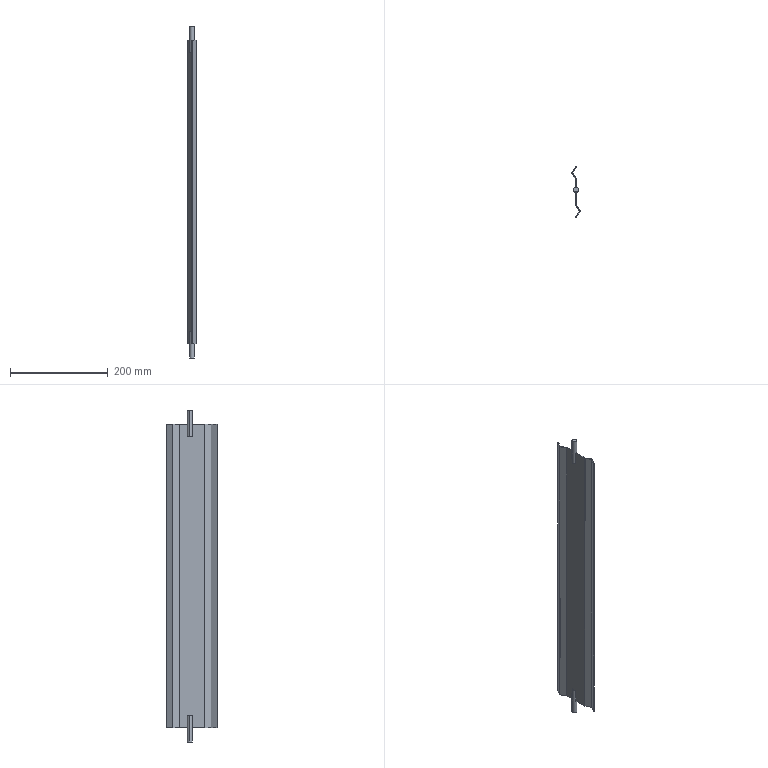Part | SolidWorks | features Extrusion 1, ICE 1, MirrorPattern 1 | 1 solid | 26 faces | box 16.5 x 104 x 678 mm | volume 111195 mm3 | plane 22 | cylinder 4 | commonest cylinder face diameters 10 x4
STEP:
#1=CARTESIAN_POINT('',(4.25,56.5,-284.));
#2=VERTEX_POINT('',#1);
#3=CARTESIAN_POINT('',(0.,61.443,-284.));
#4=VERTEX_POINT('',#3);
#5=CARTESIAN_POINT('',(-0.75,56.5,-284.));
#6=DIRECTION('',(0.,0.,1.));
#7=DIRECTION('',(1.,0.,0.));
#8=AXIS2_PLACEMENT_3D('',#5,#6,#7);
#9=CIRCLE('',#8,5.);
#10=EDGE_CURVE('',#2,#4,#9,.T.);
#11=ORIENTED_EDGE('',*,*,#10,.F.);
#12=CARTESIAN_POINT('',(4.25,56.5,-339.));
#13=VERTEX_POINT('',#12);
#14=CARTESIAN_POINT('',(4.25,56.5,-284.));
#15=DIRECTION('',(0.,0.,-1.));
#16=VECTOR('',#15,1000.);
#17=LINE('',#14,#16);
#18=EDGE_CURVE('',#2,#13,#17,.T.);
#19=ORIENTED_EDGE('',*,*,#18,.T.);
#20=CARTESIAN_POINT('',(-5.75,56.5,-339.));
#21=VERTEX_POINT('',#20);
#22=CARTESIAN_POINT('',(-0.75,56.5,-339.));
#23=DIRECTION('',(0.,0.,1.));
#24=DIRECTION('',(1.,0.,0.));
#25=AXIS2_PLACEMENT_3D('',#22,#23,#24);
#26=CIRCLE('',#25,5.);
#27=EDGE_CURVE('',#13,#21,#26,.T.);
#28=ORIENTED_EDGE('',*,*,#27,.T.);
#29=CARTESIAN_POINT('',(-5.75,56.5,-284.));
#30=VERTEX_POINT('',#29);
#31=CARTESIAN_POINT('',(-5.75,56.5,-284.));
#32=DIRECTION('',(0.,0.,-1.));
#33=VECTOR('',#32,1000.);
#34=LINE('',#31,#33);
#35=EDGE_CURVE('',#30,#21,#34,.T.);
#36=ORIENTED_EDGE('',*,*,#35,.F.);
#37=CARTESIAN_POINT('',(-1.5,61.443,-284.));
#38=VERTEX_POINT('',#37);
#39=CARTESIAN_POINT('',(-0.75,56.5,-284.));
#40=DIRECTION('',(0.,0.,1.));
#41=DIRECTION('',(1.,0.,0.));
#42=AXIS2_PLACEMENT_3D('',#39,#40,#41);
#43=CIRCLE('',#42,5.);
#44=EDGE_CURVE('',#38,#30,#43,.T.);
#45=ORIENTED_EDGE('',*,*,#44,.F.);
#46=CARTESIAN_POINT('',(-1.5,61.443,-310.));
#47=VERTEX_POINT('',#46);
#48=CARTESIAN_POINT('',(-1.5,61.443,-284.));
#49=DIRECTION('',(0.,0.,-1.));
#50=VECTOR('',#49,1000.);
#51=LINE('',#48,#50);
#52=EDGE_CURVE('',#38,#47,#51,.T.);
#53=ORIENTED_EDGE('',*,*,#52,.T.);
#54=CARTESIAN_POINT('',(0.,61.443,-310.));
#55=VERTEX_POINT('',#54);
#56=CARTESIAN_POINT('',(-0.75,56.5,-310.));
#57=DIRECTION('',(0.,0.,1.));
#58=DIRECTION('',(-1.,0.,0.));
#59=AXIS2_PLACEMENT_3D('',#56,#57,#58);
#60=CIRCLE('',#59,5.);
#61=EDGE_CURVE('',#55,#47,#60,.T.);
#62=ORIENTED_EDGE('',*,*,#61,.F.);
#63=CARTESIAN_POINT('',(0.,61.443,-284.));
#64=DIRECTION('',(0.,0.,1.));
#65=VECTOR('',#64,1000.);
#66=LINE('',#63,#65);
#67=EDGE_CURVE('',#55,#4,#66,.T.);
#68=ORIENTED_EDGE('',*,*,#67,.T.);
#69=EDGE_LOOP('',(#11,#19,#28,#36,#45,#53,#62,#68));
#70=FACE_OUTER_BOUND('',#69,.T.);
#71=CARTESIAN_POINT('',(-0.75,56.5,-284.));
#72=DIRECTION('',(0.,0.,-1.));
#73=DIRECTION('',(-1.,0.,0.));
#74=AXIS2_PLACEMENT_3D('',#71,#72,#73);
#75=CYLINDRICAL_SURFACE('',#74,5.);
#76=ADVANCED_FACE('',(#70),#75,.T.);
#77=CARTESIAN_POINT('',(-1.5,61.443,284.));
#78=VERTEX_POINT('',#77);
#79=CARTESIAN_POINT('',(-5.75,56.5,284.));
#80=VERTEX_POINT('',#79);
#81=CARTESIAN_POINT('',(-0.75,56.5,284.));
#82=DIRECTION('',(0.,0.,1.));
#83=DIRECTION('',(1.,0.,0.));
#84=AXIS2_PLACEMENT_3D('',#81,#82,#83);
#85=CIRCLE('',#84,5.);
#86=EDGE_CURVE('',#78,#80,#85,.T.);
#87=ORIENTED_EDGE('',*,*,#86,.T.);
#88=CARTESIAN_POINT('',(-5.75,56.5,339.));
#89=VERTEX_POINT('',#88);
#90=CARTESIAN_POINT('',(-5.75,56.5,284.));
#91=DIRECTION('',(0.,0.,1.));
#92=VECTOR('',#91,1000.);
#93=LINE('',#90,#92);
#94=EDGE_CURVE('',#80,#89,#93,.T.);
#95=ORIENTED_EDGE('',*,*,#94,.T.);
#96=CARTESIAN_POINT('',(4.25,56.5,339.));
#97=VERTEX_POINT('',#96);
#98=CARTESIAN_POINT('',(-0.75,56.5,339.));
#99=DIRECTION('',(0.,0.,1.));
#100=DIRECTION('',(1.,0.,0.));
#101=AXIS2_PLACEMENT_3D('',#98,#99,#100);
#102=CIRCLE('',#101,5.);
#103=EDGE_CURVE('',#97,#89,#102,.T.);
#104=ORIENTED_EDGE('',*,*,#103,.F.);
#105=CARTESIAN_POINT('',(4.25,56.5,284.));
#106=VERTEX_POINT('',#105);
#107=CARTESIAN_POINT('',(4.25,56.5,284.));
#108=DIRECTION('',(0.,0.,1.));
#109=VECTOR('',#108,1000.);
#110=LINE('',#107,#109);
#111=EDGE_CURVE('',#106,#97,#110,.T.);
#112=ORIENTED_EDGE('',*,*,#111,.F.);
#113=CARTESIAN_POINT('',(0.,61.443,284.));
#114=VERTEX_POINT('',#113);
#115=CARTESIAN_POINT('',(-0.75,56.5,284.));
#116=DIRECTION('',(0.,0.,1.));
#117=DIRECTION('',(1.,0.,0.));
#118=AXIS2_PLACEMENT_3D('',#115,#116,#117);
#119=CIRCLE('',#118,5.);
#120=EDGE_CURVE('',#106,#114,#119,.T.);
#121=ORIENTED_EDGE('',*,*,#120,.T.);
#122=CARTESIAN_POINT('',(0.,61.443,310.));
#123=VERTEX_POINT('',#122);
#124=CARTESIAN_POINT('',(0.,61.443,284.));
#125=DIRECTION('',(0.,0.,-1.));
#126=VECTOR('',#125,1000.);
#127=LINE('',#124,#126);
#128=EDGE_CURVE('',#123,#114,#127,.T.);
#129=ORIENTED_EDGE('',*,*,#128,.F.);
#130=CARTESIAN_POINT('',(-1.5,61.443,310.));
#131=VERTEX_POINT('',#130);
#132=CARTESIAN_POINT('',(-0.75,56.5,310.));
#133=DIRECTION('',(0.,0.,-1.));
#134=DIRECTION('',(-1.,0.,0.));
#135=AXIS2_PLACEMENT_3D('',#132,#133,#134);
#136=CIRCLE('',#135,5.);
#137=EDGE_CURVE('',#131,#123,#136,.T.);
#138=ORIENTED_EDGE('',*,*,#137,.F.);
#139=CARTESIAN_POINT('',(-1.5,61.443,284.));
#140=DIRECTION('',(0.,0.,1.));
#141=VECTOR('',#140,1000.);
#142=LINE('',#139,#141);
#143=EDGE_CURVE('',#78,#131,#142,.T.);
#144=ORIENTED_EDGE('',*,*,#143,.F.);
#145=EDGE_LOOP('',(#87,#95,#104,#112,#121,#129,#138,#144));
#146=FACE_OUTER_BOUND('',#145,.T.);
#147=CARTESIAN_POINT('',(-0.75,56.5,284.));
#148=DIRECTION('',(0.,0.,1.));
#149=DIRECTION('',(1.,0.,0.));
#150=AXIS2_PLACEMENT_3D('',#147,#148,#149);
#151=CYLINDRICAL_SURFACE('',#150,5.);
#152=ADVANCED_FACE('',(#146),#151,.T.);
#153=ORIENTED_EDGE('',*,*,#67,.F.);
#154=CARTESIAN_POINT('',(0.,78.421,-310.));
#155=VERTEX_POINT('',#154);
#156=CARTESIAN_POINT('',(0.,25.981,-310.));
#157=DIRECTION('',(0.,1.,0.));
#158=VECTOR('',#157,1000.);
#159=LINE('',#156,#158);
#160=EDGE_CURVE('',#55,#155,#159,.T.);
#161=ORIENTED_EDGE('',*,*,#160,.T.);
#162=CARTESIAN_POINT('',(0.,78.421,310.));
#163=VERTEX_POINT('',#162);
#164=CARTESIAN_POINT('',(0.,78.421,310.));
#165=DIRECTION('',(0.,0.,-1.));
#166=VECTOR('',#165,1000.);
#167=LINE('',#164,#166);
#168=EDGE_CURVE('',#163,#155,#167,.T.);
#169=ORIENTED_EDGE('',*,*,#168,.F.);
#170=CARTESIAN_POINT('',(0.,25.981,310.));
#171=DIRECTION('',(0.,1.,0.));
#172=VECTOR('',#171,1000.);
#173=LINE('',#170,#172);
#174=EDGE_CURVE('',#123,#163,#173,.T.);
#175=ORIENTED_EDGE('',*,*,#174,.F.);
#176=ORIENTED_EDGE('',*,*,#128,.T.);
#177=CARTESIAN_POINT('',(0.,51.557,284.));
#178=VERTEX_POINT('',#177);
#179=CARTESIAN_POINT('',(0.,25.981,284.));
#180=DIRECTION('',(0.,1.,0.));
#181=VECTOR('',#180,1000.);
#182=LINE('',#179,#181);
#183=EDGE_CURVE('',#178,#114,#182,.T.);
#184=ORIENTED_EDGE('',*,*,#183,.F.);
#185=CARTESIAN_POINT('',(0.,51.557,310.));
#186=VERTEX_POINT('',#185);
#187=CARTESIAN_POINT('',(0.,51.557,284.));
#188=DIRECTION('',(0.,0.,1.));
#189=VECTOR('',#188,1000.);
#190=LINE('',#187,#189);
#191=EDGE_CURVE('',#178,#186,#190,.T.);
#192=ORIENTED_EDGE('',*,*,#191,.T.);
#193=CARTESIAN_POINT('',(0.,25.981,310.));
#194=VERTEX_POINT('',#193);
#195=CARTESIAN_POINT('',(0.,25.981,310.));
#196=DIRECTION('',(0.,1.,0.));
#197=VECTOR('',#196,1000.);
#198=LINE('',#195,#197);
#199=EDGE_CURVE('',#194,#186,#198,.T.);
#200=ORIENTED_EDGE('',*,*,#199,.F.);
#201=CARTESIAN_POINT('',(0.,25.981,-310.));
#202=VERTEX_POINT('',#201);
#203=CARTESIAN_POINT('',(0.,25.981,310.));
#204=DIRECTION('',(0.,0.,-1.));
#205=VECTOR('',#204,1000.);
#206=LINE('',#203,#205);
#207=EDGE_CURVE('',#194,#202,#206,.T.);
#208=ORIENTED_EDGE('',*,*,#207,.T.);
#209=CARTESIAN_POINT('',(0.,51.557,-310.));
#210=VERTEX_POINT('',#209);
#211=CARTESIAN_POINT('',(0.,25.981,-310.));
#212=DIRECTION('',(0.,1.,0.));
#213=VECTOR('',#212,1000.);
#214=LINE('',#211,#213);
#215=EDGE_CURVE('',#202,#210,#214,.T.);
#216=ORIENTED_EDGE('',*,*,#215,.T.);
#217=CARTESIAN_POINT('',(0.,51.557,-284.));
#218=VERTEX_POINT('',#217);
#219=CARTESIAN_POINT('',(0.,51.557,-284.));
#220=DIRECTION('',(0.,0.,-1.));
#221=VECTOR('',#220,1000.);
#222=LINE('',#219,#221);
#223=EDGE_CURVE('',#218,#210,#222,.T.);
#224=ORIENTED_EDGE('',*,*,#223,.F.);
#225=CARTESIAN_POINT('',(0.,25.981,-284.));
#226=DIRECTION('',(0.,-1.,0.));
#227=VECTOR('',#226,1000.);
#228=LINE('',#225,#227);
#229=EDGE_CURVE('',#4,#218,#228,.T.);
#230=ORIENTED_EDGE('',*,*,#229,.F.);
#231=EDGE_LOOP('',(#153,#161,#169,#175,#176,#184,#192,#200,#208,#216,#224,#230));
#232=FACE_OUTER_BOUND('',#231,.T.);
#233=CARTESIAN_POINT('',(0.,25.981,310.));
#234=DIRECTION('',(-1.,0.,0.));
#235=DIRECTION('',(0.,-1.,0.));
#236=AXIS2_PLACEMENT_3D('',#233,#234,#235);
#237=PLANE('',#236);
#238=ADVANCED_FACE('',(#232),#237,.F.);
#239=CARTESIAN_POINT('',(-1.5,51.557,-310.));
#240=VERTEX_POINT('',#239);
#241=CARTESIAN_POINT('',(-1.5,51.557,-284.));
#242=VERTEX_POINT('',#241);
#243=CARTESIAN_POINT('',(-1.5,51.557,-284.));
#244=DIRECTION('',(0.,0.,1.));
#245=VECTOR('',#244,1000.);
#246=LINE('',#243,#245);
#247=EDGE_CURVE('',#240,#242,#246,.T.);
#248=ORIENTED_EDGE('',*,*,#247,.F.);
#249=CARTESIAN_POINT('',(-1.5,25.579,-310.));
#250=VERTEX_POINT('',#249);
#251=CARTESIAN_POINT('',(-1.5,25.579,-310.));
#252=DIRECTION('',(0.,-1.,0.));
#253=VECTOR('',#252,1000.);
#254=LINE('',#251,#253);
#255=EDGE_CURVE('',#240,#250,#254,.T.);
#256=ORIENTED_EDGE('',*,*,#255,.T.);
#257=CARTESIAN_POINT('',(-1.5,25.579,310.));
#258=VERTEX_POINT('',#257);
#259=CARTESIAN_POINT('',(-1.5,25.579,310.));
#260=DIRECTION('',(0.,0.,-1.));
#261=VECTOR('',#260,1000.);
#262=LINE('',#259,#261);
#263=EDGE_CURVE('',#258,#250,#262,.T.);
#264=ORIENTED_EDGE('',*,*,#263,.F.);
#265=CARTESIAN_POINT('',(-1.5,51.557,310.));
#266=VERTEX_POINT('',#265);
#267=CARTESIAN_POINT('',(-1.5,25.579,310.));
#268=DIRECTION('',(0.,-1.,0.));
#269=VECTOR('',#268,1000.);
#270=LINE('',#267,#269);
#271=EDGE_CURVE('',#266,#258,#270,.T.);
#272=ORIENTED_EDGE('',*,*,#271,.F.);
#273=CARTESIAN_POINT('',(-1.5,51.557,284.));
#274=VERTEX_POINT('',#273);
#275=CARTESIAN_POINT('',(-1.5,51.557,284.));
#276=DIRECTION('',(0.,0.,-1.));
#277=VECTOR('',#276,1000.);
#278=LINE('',#275,#277);
#279=EDGE_CURVE('',#266,#274,#278,.T.);
#280=ORIENTED_EDGE('',*,*,#279,.T.);
#281=CARTESIAN_POINT('',(-1.5,25.579,284.));
#282=DIRECTION('',(0.,-1.,0.));
#283=VECTOR('',#282,1000.);
#284=LINE('',#281,#283);
#285=EDGE_CURVE('',#78,#274,#284,.T.);
#286=ORIENTED_EDGE('',*,*,#285,.F.);
#287=ORIENTED_EDGE('',*,*,#143,.T.);
#288=CARTESIAN_POINT('',(-1.5,78.019,310.));
#289=VERTEX_POINT('',#288);
#290=CARTESIAN_POINT('',(-1.5,25.579,310.));
#291=DIRECTION('',(0.,-1.,0.));
#292=VECTOR('',#291,1000.);
#293=LINE('',#290,#292);
#294=EDGE_CURVE('',#289,#131,#293,.T.);
#295=ORIENTED_EDGE('',*,*,#294,.F.);
#296=CARTESIAN_POINT('',(-1.5,78.019,-310.));
#297=VERTEX_POINT('',#296);
#298=CARTESIAN_POINT('',(-1.5,78.019,310.));
#299=DIRECTION('',(0.,0.,-1.));
#300=VECTOR('',#299,1000.);
#301=LINE('',#298,#300);
#302=EDGE_CURVE('',#289,#297,#301,.T.);
#303=ORIENTED_EDGE('',*,*,#302,.T.);
#304=CARTESIAN_POINT('',(-1.5,25.579,-310.));
#305=DIRECTION('',(0.,-1.,0.));
#306=VECTOR('',#305,1000.);
#307=LINE('',#304,#306);
#308=EDGE_CURVE('',#297,#47,#307,.T.);
#309=ORIENTED_EDGE('',*,*,#308,.T.);
#310=ORIENTED_EDGE('',*,*,#52,.F.);
#311=CARTESIAN_POINT('',(-1.5,25.579,-284.));
#312=DIRECTION('',(0.,1.,0.));
#313=VECTOR('',#312,1000.);
#314=LINE('',#311,#313);
#315=EDGE_CURVE('',#242,#38,#314,.T.);
#316=ORIENTED_EDGE('',*,*,#315,.F.);
#317=EDGE_LOOP('',(#248,#256,#264,#272,#280,#286,#287,#295,#303,#309,#310,#316));
#318=FACE_OUTER_BOUND('',#317,.T.);
#319=CARTESIAN_POINT('',(-1.5,25.579,310.));
#320=DIRECTION('',(1.,0.,0.));
#321=DIRECTION('',(0.,0.,-1.));
#322=AXIS2_PLACEMENT_3D('',#319,#320,#321);
#323=PLANE('',#322);
#324=ADVANCED_FACE('',(#318),#323,.F.);
#325=ORIENTED_EDGE('',*,*,#255,.F.);
#326=CARTESIAN_POINT('',(-0.75,56.5,-310.));
#327=DIRECTION('',(0.,0.,1.));
#328=DIRECTION('',(-1.,0.,0.));
#329=AXIS2_PLACEMENT_3D('',#326,#327,#328);
#330=CIRCLE('',#329,5.);
#331=EDGE_CURVE('',#240,#210,#330,.T.);
#332=ORIENTED_EDGE('',*,*,#331,.T.);
#333=ORIENTED_EDGE('',*,*,#215,.F.);
#334=CARTESIAN_POINT('',(7.5,12.99,-310.));
#335=VERTEX_POINT('',#334);
#336=CARTESIAN_POINT('',(7.5,12.99,-310.));
#337=DIRECTION('',(-0.5,0.866,0.));
#338=VECTOR('',#337,1000.);
#339=LINE('',#336,#338);
#340=EDGE_CURVE('',#335,#202,#339,.T.);
#341=ORIENTED_EDGE('',*,*,#340,.F.);
#342=CARTESIAN_POINT('',(0.,0.,-310.));
#343=VERTEX_POINT('',#342);
#344=CARTESIAN_POINT('',(0.,0.,-310.));
#345=DIRECTION('',(0.5,0.866,0.));
#346=VECTOR('',#345,1000.);
#347=LINE('',#344,#346);
#348=EDGE_CURVE('',#343,#335,#347,.T.);
#349=ORIENTED_EDGE('',*,*,#348,.F.);
#350=CARTESIAN_POINT('',(-1.299,0.75,-310.));
#351=VERTEX_POINT('',#350);
#352=CARTESIAN_POINT('',(0.,0.,-310.));
#353=DIRECTION('',(0.866,-0.5,0.));
#354=VECTOR('',#353,1000.);
#355=LINE('',#352,#354);
#356=EDGE_CURVE('',#351,#343,#355,.T.);
#357=ORIENTED_EDGE('',*,*,#356,.F.);
#358=CARTESIAN_POINT('',(5.768,12.99,-310.));
#359=VERTEX_POINT('',#358);
#360=CARTESIAN_POINT('',(-1.299,0.75,-310.));
#361=DIRECTION('',(-0.5,-0.866,0.));
#362=VECTOR('',#361,1000.);
#363=LINE('',#360,#362);
#364=EDGE_CURVE('',#359,#351,#363,.T.);
#365=ORIENTED_EDGE('',*,*,#364,.F.);
#366=CARTESIAN_POINT('',(5.768,12.99,-310.));
#367=DIRECTION('',(0.5,-0.866,0.));
#368=VECTOR('',#367,1000.);
#369=LINE('',#366,#368);
#370=EDGE_CURVE('',#250,#359,#369,.T.);
#371=ORIENTED_EDGE('',*,*,#370,.F.);
#372=EDGE_LOOP('',(#325,#332,#333,#341,#349,#357,#365,#371));
#373=FACE_OUTER_BOUND('',#372,.T.);
#374=CARTESIAN_POINT('',(0.,0.,-310.));
#375=DIRECTION('',(0.,0.,-1.));
#376=DIRECTION('',(-1.,0.,0.));
#377=AXIS2_PLACEMENT_3D('',#374,#375,#376);
#378=PLANE('',#377);
#379=ADVANCED_FACE('',(#373),#378,.T.);
#380=ORIENTED_EDGE('',*,*,#294,.T.);
#381=ORIENTED_EDGE('',*,*,#137,.T.);
#382=ORIENTED_EDGE('',*,*,#174,.T.);
#383=CARTESIAN_POINT('',(-7.268,91.01,310.));
#384=VERTEX_POINT('',#383);
#385=CARTESIAN_POINT('',(0.,78.421,310.));
#386=DIRECTION('',(-0.5,0.866,0.));
#387=VECTOR('',#386,1000.);
#388=LINE('',#385,#387);
#389=EDGE_CURVE('',#163,#384,#388,.T.);
#390=ORIENTED_EDGE('',*,*,#389,.T.);
#391=CARTESIAN_POINT('',(-0.201,103.25,310.));
#392=VERTEX_POINT('',#391);
#393=CARTESIAN_POINT('',(-7.268,91.01,310.));
#394=DIRECTION('',(0.5,0.866,0.));
#395=VECTOR('',#394,1000.);
#396=LINE('',#393,#395);
#397=EDGE_CURVE('',#384,#392,#396,.T.);
#398=ORIENTED_EDGE('',*,*,#397,.T.);
#399=CARTESIAN_POINT('',(-1.5,104.,310.));
#400=VERTEX_POINT('',#399);
#401=CARTESIAN_POINT('',(-0.201,103.25,310.));
#402=DIRECTION('',(-0.866,0.5,0.));
#403=VECTOR('',#402,1000.);
#404=LINE('',#401,#403);
#405=EDGE_CURVE('',#392,#400,#404,.T.);
#406=ORIENTED_EDGE('',*,*,#405,.T.);
#407=CARTESIAN_POINT('',(-9.,91.01,310.));
#408=VERTEX_POINT('',#407);
#409=CARTESIAN_POINT('',(-9.,91.01,310.));
#410=DIRECTION('',(-0.5,-0.866,0.));
#411=VECTOR('',#410,1000.);
#412=LINE('',#409,#411);
#413=EDGE_CURVE('',#400,#408,#412,.T.);
#414=ORIENTED_EDGE('',*,*,#413,.T.);
#415=CARTESIAN_POINT('',(-1.5,78.019,310.));
#416=DIRECTION('',(0.5,-0.866,0.));
#417=VECTOR('',#416,1000.);
#418=LINE('',#415,#417);
#419=EDGE_CURVE('',#408,#289,#418,.T.);
#420=ORIENTED_EDGE('',*,*,#419,.T.);
#421=EDGE_LOOP('',(#380,#381,#382,#390,#398,#406,#414,#420));
#422=FACE_OUTER_BOUND('',#421,.T.);
#423=CARTESIAN_POINT('',(0.,0.,310.));
#424=DIRECTION('',(0.,0.,-1.));
#425=DIRECTION('',(-1.,0.,0.));
#426=AXIS2_PLACEMENT_3D('',#423,#424,#425);
#427=PLANE('',#426);
#428=ADVANCED_FACE('',(#422),#427,.F.);
#429=ORIENTED_EDGE('',*,*,#356,.T.);
#430=CARTESIAN_POINT('',(0.,0.,310.));
#431=VERTEX_POINT('',#430);
#432=CARTESIAN_POINT('',(0.,0.,310.));
#433=DIRECTION('',(0.,0.,-1.));
#434=VECTOR('',#433,1000.);
#435=LINE('',#432,#434);
#436=EDGE_CURVE('',#431,#343,#435,.T.);
#437=ORIENTED_EDGE('',*,*,#436,.F.);
#438=CARTESIAN_POINT('',(-1.299,0.75,310.));
#439=VERTEX_POINT('',#438);
#440=CARTESIAN_POINT('',(0.,0.,310.));
#441=DIRECTION('',(0.866,-0.5,0.));
#442=VECTOR('',#441,1000.);
#443=LINE('',#440,#442);
#444=EDGE_CURVE('',#439,#431,#443,.T.);
#445=ORIENTED_EDGE('',*,*,#444,.F.);
#446=CARTESIAN_POINT('',(-1.299,0.75,310.));
#447=DIRECTION('',(0.,0.,-1.));
#448=VECTOR('',#447,1000.);
#449=LINE('',#446,#448);
#450=EDGE_CURVE('',#439,#351,#449,.T.);
#451=ORIENTED_EDGE('',*,*,#450,.T.);
#452=EDGE_LOOP('',(#429,#437,#445,#451));
#453=FACE_OUTER_BOUND('',#452,.T.);
#454=CARTESIAN_POINT('',(0.,0.,310.));
#455=DIRECTION('',(0.5,0.866,0.));
#456=DIRECTION('',(-0.866,0.5,0.));
#457=AXIS2_PLACEMENT_3D('',#454,#455,#456);
#458=PLANE('',#457);
#459=ADVANCED_FACE('',(#453),#458,.F.);
#460=ORIENTED_EDGE('',*,*,#348,.T.);
#461=CARTESIAN_POINT('',(7.5,12.99,310.));
#462=VERTEX_POINT('',#461);
#463=CARTESIAN_POINT('',(7.5,12.99,310.));
#464=DIRECTION('',(0.,0.,-1.));
#465=VECTOR('',#464,1000.);
#466=LINE('',#463,#465);
#467=EDGE_CURVE('',#462,#335,#466,.T.);
#468=ORIENTED_EDGE('',*,*,#467,.F.);
#469=CARTESIAN_POINT('',(0.,0.,310.));
#470=DIRECTION('',(0.5,0.866,0.));
#471=VECTOR('',#470,1000.);
#472=LINE('',#469,#471);
#473=EDGE_CURVE('',#431,#462,#472,.T.);
#474=ORIENTED_EDGE('',*,*,#473,.F.);
#475=ORIENTED_EDGE('',*,*,#436,.T.);
#476=EDGE_LOOP('',(#460,#468,#474,#475));
#477=FACE_OUTER_BOUND('',#476,.T.);
#478=CARTESIAN_POINT('',(0.,0.,310.));
#479=DIRECTION('',(-0.866,0.5,0.));
#480=DIRECTION('',(-0.5,-0.866,0.));
#481=AXIS2_PLACEMENT_3D('',#478,#479,#480);
#482=PLANE('',#481);
#483=ADVANCED_FACE('',(#477),#482,.F.);
#484=ORIENTED_EDGE('',*,*,#340,.T.);
#485=ORIENTED_EDGE('',*,*,#207,.F.);
#486=CARTESIAN_POINT('',(7.5,12.99,310.));
#487=DIRECTION('',(-0.5,0.866,0.));
#488=VECTOR('',#487,1000.);
#489=LINE('',#486,#488);
#490=EDGE_CURVE('',#462,#194,#489,.T.);
#491=ORIENTED_EDGE('',*,*,#490,.F.);
#492=ORIENTED_EDGE('',*,*,#467,.T.);
#493=EDGE_LOOP('',(#484,#485,#491,#492));
#494=FACE_OUTER_BOUND('',#493,.T.);
#495=CARTESIAN_POINT('',(7.5,12.99,310.));
#496=DIRECTION('',(-0.866,-0.5,0.));
#497=DIRECTION('',(0.5,-0.866,0.));
#498=AXIS2_PLACEMENT_3D('',#495,#496,#497);
#499=PLANE('',#498);
#500=ADVANCED_FACE('',(#494),#499,.F.);
#501=CARTESIAN_POINT('',(-7.268,91.01,-310.));
#502=VERTEX_POINT('',#501);
#503=CARTESIAN_POINT('',(0.,78.421,-310.));
#504=DIRECTION('',(-0.5,0.866,0.));
#505=VECTOR('',#504,1000.);
#506=LINE('',#503,#505);
#507=EDGE_CURVE('',#155,#502,#506,.T.);
#508=ORIENTED_EDGE('',*,*,#507,.T.);
#509=CARTESIAN_POINT('',(-7.268,91.01,310.));
#510=DIRECTION('',(0.,0.,-1.));
#511=VECTOR('',#510,1000.);
#512=LINE('',#509,#511);
#513=EDGE_CURVE('',#384,#502,#512,.T.);
#514=ORIENTED_EDGE('',*,*,#513,.F.);
#515=ORIENTED_EDGE('',*,*,#389,.F.);
#516=ORIENTED_EDGE('',*,*,#168,.T.);
#517=EDGE_LOOP('',(#508,#514,#515,#516));
#518=FACE_OUTER_BOUND('',#517,.T.);
#519=CARTESIAN_POINT('',(0.,78.421,310.));
#520=DIRECTION('',(-0.866,-0.5,0.));
#521=DIRECTION('',(0.5,-0.866,0.));
#522=AXIS2_PLACEMENT_3D('',#519,#520,#521);
#523=PLANE('',#522);
#524=ADVANCED_FACE('',(#518),#523,.F.);
#525=CARTESIAN_POINT('',(-0.201,103.25,-310.));
#526=VERTEX_POINT('',#525);
#527=CARTESIAN_POINT('',(-7.268,91.01,-310.));
#528=DIRECTION('',(0.5,0.866,0.));
#529=VECTOR('',#528,1000.);
#530=LINE('',#527,#529);
#531=EDGE_CURVE('',#502,#526,#530,.T.);
#532=ORIENTED_EDGE('',*,*,#531,.T.);
#533=CARTESIAN_POINT('',(-0.201,103.25,310.));
#534=DIRECTION('',(0.,0.,-1.));
#535=VECTOR('',#534,1000.);
#536=LINE('',#533,#535);
#537=EDGE_CURVE('',#392,#526,#536,.T.);
#538=ORIENTED_EDGE('',*,*,#537,.F.);
#539=ORIENTED_EDGE('',*,*,#397,.F.);
#540=ORIENTED_EDGE('',*,*,#513,.T.);
#541=EDGE_LOOP('',(#532,#538,#539,#540));
#542=FACE_OUTER_BOUND('',#541,.T.);
#543=CARTESIAN_POINT('',(-7.268,91.01,310.));
#544=DIRECTION('',(-0.866,0.5,0.));
#545=DIRECTION('',(-0.5,-0.866,0.));
#546=AXIS2_PLACEMENT_3D('',#543,#544,#545);
#547=PLANE('',#546);
#548=ADVANCED_FACE('',(#542),#547,.F.);
#549=CARTESIAN_POINT('',(-1.5,104.,-310.));
#550=VERTEX_POINT('',#549);
#551=CARTESIAN_POINT('',(-0.201,103.25,-310.));
#552=DIRECTION('',(-0.866,0.5,0.));
#553=VECTOR('',#552,1000.);
#554=LINE('',#551,#553);
#555=EDGE_CURVE('',#526,#550,#554,.T.);
#556=ORIENTED_EDGE('',*,*,#555,.T.);
#557=CARTESIAN_POINT('',(-1.5,104.,310.));
#558=DIRECTION('',(0.,0.,-1.));
#559=VECTOR('',#558,1000.);
#560=LINE('',#557,#559);
#561=EDGE_CURVE('',#400,#550,#560,.T.);
#562=ORIENTED_EDGE('',*,*,#561,.F.);
#563=ORIENTED_EDGE('',*,*,#405,.F.);
#564=ORIENTED_EDGE('',*,*,#537,.T.);
#565=EDGE_LOOP('',(#556,#562,#563,#564));
#566=FACE_OUTER_BOUND('',#565,.T.);
#567=CARTESIAN_POINT('',(-0.201,103.25,310.));
#568=DIRECTION('',(-0.5,-0.866,0.));
#569=DIRECTION('',(0.866,-0.5,0.));
#570=AXIS2_PLACEMENT_3D('',#567,#568,#569);
#571=PLANE('',#570);
#572=ADVANCED_FACE('',(#566),#571,.F.);
#573=CARTESIAN_POINT('',(-9.,91.01,-310.));
#574=VERTEX_POINT('',#573);
#575=CARTESIAN_POINT('',(-9.,91.01,-310.));
#576=DIRECTION('',(-0.5,-0.866,0.));
#577=VECTOR('',#576,1000.);
#578=LINE('',#575,#577);
#579=EDGE_CURVE('',#550,#574,#578,.T.);
#580=ORIENTED_EDGE('',*,*,#579,.T.);
#581=CARTESIAN_POINT('',(-9.,91.01,310.));
#582=DIRECTION('',(0.,0.,-1.));
#583=VECTOR('',#582,1000.);
#584=LINE('',#581,#583);
#585=EDGE_CURVE('',#408,#574,#584,.T.);
#586=ORIENTED_EDGE('',*,*,#585,.F.);
#587=ORIENTED_EDGE('',*,*,#413,.F.);
#588=ORIENTED_EDGE('',*,*,#561,.T.);
#589=EDGE_LOOP('',(#580,#586,#587,#588));
#590=FACE_OUTER_BOUND('',#589,.T.);
#591=CARTESIAN_POINT('',(-9.,91.01,310.));
#592=DIRECTION('',(0.866,-0.5,0.));
#593=DIRECTION('',(0.5,0.866,0.));
#594=AXIS2_PLACEMENT_3D('',#591,#592,#593);
#595=PLANE('',#594);
#596=ADVANCED_FACE('',(#590),#595,.F.);
#597=CARTESIAN_POINT('',(-1.5,78.019,-310.));
#598=DIRECTION('',(0.5,-0.866,0.));
#599=VECTOR('',#598,1000.);
#600=LINE('',#597,#599);
#601=EDGE_CURVE('',#574,#297,#600,.T.);
#602=ORIENTED_EDGE('',*,*,#601,.T.);
#603=ORIENTED_EDGE('',*,*,#302,.F.);
#604=ORIENTED_EDGE('',*,*,#419,.F.);
#605=ORIENTED_EDGE('',*,*,#585,.T.);
#606=EDGE_LOOP('',(#602,#603,#604,#605));
#607=FACE_OUTER_BOUND('',#606,.T.);
#608=CARTESIAN_POINT('',(-1.5,78.019,310.));
#609=DIRECTION('',(0.866,0.5,0.));
#610=DIRECTION('',(-0.5,0.866,0.));
#611=AXIS2_PLACEMENT_3D('',#608,#609,#610);
#612=PLANE('',#611);
#613=ADVANCED_FACE('',(#607),#612,.F.);
#614=ORIENTED_EDGE('',*,*,#370,.T.);
#615=CARTESIAN_POINT('',(5.768,12.99,310.));
#616=VERTEX_POINT('',#615);
#617=CARTESIAN_POINT('',(5.768,12.99,310.));
#618=DIRECTION('',(0.,0.,-1.));
#619=VECTOR('',#618,1000.);
#620=LINE('',#617,#619);
#621=EDGE_CURVE('',#616,#359,#620,.T.);
#622=ORIENTED_EDGE('',*,*,#621,.F.);
#623=CARTESIAN_POINT('',(5.768,12.99,310.));
#624=DIRECTION('',(0.5,-0.866,0.));
#625=VECTOR('',#624,1000.);
#626=LINE('',#623,#625);
#627=EDGE_CURVE('',#258,#616,#626,.T.);
#628=ORIENTED_EDGE('',*,*,#627,.F.);
#629=ORIENTED_EDGE('',*,*,#263,.T.);
#630=EDGE_LOOP('',(#614,#622,#628,#629));
#631=FACE_OUTER_BOUND('',#630,.T.);
#632=CARTESIAN_POINT('',(5.768,12.99,310.));
#633=DIRECTION('',(0.866,0.5,0.));
#634=DIRECTION('',(-0.5,0.866,0.));
#635=AXIS2_PLACEMENT_3D('',#632,#633,#634);
#636=PLANE('',#635);
#637=ADVANCED_FACE('',(#631),#636,.F.);
#638=ORIENTED_EDGE('',*,*,#364,.T.);
#639=ORIENTED_EDGE('',*,*,#450,.F.);
#640=CARTESIAN_POINT('',(-1.299,0.75,310.));
#641=DIRECTION('',(-0.5,-0.866,0.));
#642=VECTOR('',#641,1000.);
#643=LINE('',#640,#642);
#644=EDGE_CURVE('',#616,#439,#643,.T.);
#645=ORIENTED_EDGE('',*,*,#644,.F.);
#646=ORIENTED_EDGE('',*,*,#621,.T.);
#647=EDGE_LOOP('',(#638,#639,#645,#646));
#648=FACE_OUTER_BOUND('',#647,.T.);
#649=CARTESIAN_POINT('',(-1.299,0.75,310.));
#650=DIRECTION('',(0.866,-0.5,0.));
#651=DIRECTION('',(0.5,0.866,0.));
#652=AXIS2_PLACEMENT_3D('',#649,#650,#651);
#653=PLANE('',#652);
#654=ADVANCED_FACE('',(#648),#653,.F.);
#655=ORIENTED_EDGE('',*,*,#199,.T.);
#656=CARTESIAN_POINT('',(-0.75,56.5,310.));
#657=DIRECTION('',(0.,0.,-1.));
#658=DIRECTION('',(-1.,0.,0.));
#659=AXIS2_PLACEMENT_3D('',#656,#657,#658);
#660=CIRCLE('',#659,5.);
#661=EDGE_CURVE('',#186,#266,#660,.T.);
#662=ORIENTED_EDGE('',*,*,#661,.T.);
#663=ORIENTED_EDGE('',*,*,#271,.T.);
#664=ORIENTED_EDGE('',*,*,#627,.T.);
#665=ORIENTED_EDGE('',*,*,#644,.T.);
#666=ORIENTED_EDGE('',*,*,#444,.T.);
#667=ORIENTED_EDGE('',*,*,#473,.T.);
#668=ORIENTED_EDGE('',*,*,#490,.T.);
#669=EDGE_LOOP('',(#655,#662,#663,#664,#665,#666,#667,#668));
#670=FACE_OUTER_BOUND('',#669,.T.);
#671=CARTESIAN_POINT('',(0.,0.,310.));
#672=DIRECTION('',(0.,0.,-1.));
#673=DIRECTION('',(-1.,0.,0.));
#674=AXIS2_PLACEMENT_3D('',#671,#672,#673);
#675=PLANE('',#674);
#676=ADVANCED_FACE('',(#670),#675,.F.);
#677=ORIENTED_EDGE('',*,*,#160,.F.);
#678=ORIENTED_EDGE('',*,*,#61,.T.);
#679=ORIENTED_EDGE('',*,*,#308,.F.);
#680=ORIENTED_EDGE('',*,*,#601,.F.);
#681=ORIENTED_EDGE('',*,*,#579,.F.);
#682=ORIENTED_EDGE('',*,*,#555,.F.);
#683=ORIENTED_EDGE('',*,*,#531,.F.);
#684=ORIENTED_EDGE('',*,*,#507,.F.);
#685=EDGE_LOOP('',(#677,#678,#679,#680,#681,#682,#683,#684));
#686=FACE_OUTER_BOUND('',#685,.T.);
#687=CARTESIAN_POINT('',(0.,0.,-310.));
#688=DIRECTION('',(0.,0.,-1.));
#689=DIRECTION('',(-1.,0.,0.));
#690=AXIS2_PLACEMENT_3D('',#687,#688,#689);
#691=PLANE('',#690);
#692=ADVANCED_FACE('',(#686),#691,.T.);
#693=CARTESIAN_POINT('',(-0.75,56.5,284.));
#694=DIRECTION('',(0.,0.,1.));
#695=DIRECTION('',(1.,0.,0.));
#696=AXIS2_PLACEMENT_3D('',#693,#694,#695);
#697=CIRCLE('',#696,5.);
#698=EDGE_CURVE('',#178,#106,#697,.T.);
#699=ORIENTED_EDGE('',*,*,#698,.F.);
#700=ORIENTED_EDGE('',*,*,#183,.T.);
#701=ORIENTED_EDGE('',*,*,#120,.F.);
#702=EDGE_LOOP('',(#699,#700,#701));
#703=FACE_OUTER_BOUND('',#702,.T.);
#704=CARTESIAN_POINT('',(-0.75,56.5,284.));
#705=DIRECTION('',(0.,0.,1.));
#706=DIRECTION('',(1.,0.,0.));
#707=AXIS2_PLACEMENT_3D('',#704,#705,#706);
#708=PLANE('',#707);
#709=ADVANCED_FACE('',(#703),#708,.F.);
#710=ORIENTED_EDGE('',*,*,#86,.F.);
#711=ORIENTED_EDGE('',*,*,#285,.T.);
#712=CARTESIAN_POINT('',(-0.75,56.5,284.));
#713=DIRECTION('',(0.,0.,1.));
#714=DIRECTION('',(1.,0.,0.));
#715=AXIS2_PLACEMENT_3D('',#712,#713,#714);
#716=CIRCLE('',#715,5.);
#717=EDGE_CURVE('',#80,#274,#716,.T.);
#718=ORIENTED_EDGE('',*,*,#717,.F.);
#719=EDGE_LOOP('',(#710,#711,#718));
#720=FACE_OUTER_BOUND('',#719,.T.);
#721=CARTESIAN_POINT('',(-0.75,56.5,284.));
#722=DIRECTION('',(0.,0.,1.));
#723=DIRECTION('',(1.,0.,0.));
#724=AXIS2_PLACEMENT_3D('',#721,#722,#723);
#725=PLANE('',#724);
#726=ADVANCED_FACE('',(#720),#725,.F.);
#727=ORIENTED_EDGE('',*,*,#94,.F.);
#728=ORIENTED_EDGE('',*,*,#717,.T.);
#729=ORIENTED_EDGE('',*,*,#279,.F.);
#730=ORIENTED_EDGE('',*,*,#661,.F.);
#731=ORIENTED_EDGE('',*,*,#191,.F.);
#732=ORIENTED_EDGE('',*,*,#698,.T.);
#733=ORIENTED_EDGE('',*,*,#111,.T.);
#734=CARTESIAN_POINT('',(-0.75,56.5,339.));
#735=DIRECTION('',(0.,0.,1.));
#736=DIRECTION('',(1.,0.,0.));
#737=AXIS2_PLACEMENT_3D('',#734,#735,#736);
#738=CIRCLE('',#737,5.);
#739=EDGE_CURVE('',#89,#97,#738,.T.);
#740=ORIENTED_EDGE('',*,*,#739,.F.);
#741=EDGE_LOOP('',(#727,#728,#729,#730,#731,#732,#733,#740));
#742=FACE_OUTER_BOUND('',#741,.T.);
#743=CARTESIAN_POINT('',(-0.75,56.5,284.));
#744=DIRECTION('',(0.,0.,1.));
#745=DIRECTION('',(1.,0.,0.));
#746=AXIS2_PLACEMENT_3D('',#743,#744,#745);
#747=CYLINDRICAL_SURFACE('',#746,5.);
#748=ADVANCED_FACE('',(#742),#747,.T.);
#749=ORIENTED_EDGE('',*,*,#103,.T.);
#750=ORIENTED_EDGE('',*,*,#739,.T.);
#751=EDGE_LOOP('',(#749,#750));
#752=FACE_OUTER_BOUND('',#751,.T.);
#753=CARTESIAN_POINT('',(-0.75,56.5,339.));
#754=DIRECTION('',(0.,0.,1.));
#755=DIRECTION('',(1.,0.,0.));
#756=AXIS2_PLACEMENT_3D('',#753,#754,#755);
#757=PLANE('',#756);
#758=ADVANCED_FACE('',(#752),#757,.T.);
#759=CARTESIAN_POINT('',(-0.75,56.5,-284.));
#760=DIRECTION('',(0.,0.,1.));
#761=DIRECTION('',(1.,0.,0.));
#762=AXIS2_PLACEMENT_3D('',#759,#760,#761);
#763=CIRCLE('',#762,5.);
#764=EDGE_CURVE('',#218,#2,#763,.T.);
#765=ORIENTED_EDGE('',*,*,#764,.T.);
#766=ORIENTED_EDGE('',*,*,#10,.T.);
#767=ORIENTED_EDGE('',*,*,#229,.T.);
#768=EDGE_LOOP('',(#765,#766,#767));
#769=FACE_OUTER_BOUND('',#768,.T.);
#770=CARTESIAN_POINT('',(-0.75,56.5,-284.));
#771=DIRECTION('',(0.,0.,-1.));
#772=DIRECTION('',(1.,0.,0.));
#773=AXIS2_PLACEMENT_3D('',#770,#771,#772);
#774=PLANE('',#773);
#775=ADVANCED_FACE('',(#769),#774,.F.);
#776=ORIENTED_EDGE('',*,*,#44,.T.);
#777=CARTESIAN_POINT('',(-0.75,56.5,-284.));
#778=DIRECTION('',(0.,0.,1.));
#779=DIRECTION('',(1.,0.,0.));
#780=AXIS2_PLACEMENT_3D('',#777,#778,#779);
#781=CIRCLE('',#780,5.);
#782=EDGE_CURVE('',#30,#242,#781,.T.);
#783=ORIENTED_EDGE('',*,*,#782,.T.);
#784=ORIENTED_EDGE('',*,*,#315,.T.);
#785=EDGE_LOOP('',(#776,#783,#784));
#786=FACE_OUTER_BOUND('',#785,.T.);
#787=CARTESIAN_POINT('',(-0.75,56.5,-284.));
#788=DIRECTION('',(0.,0.,-1.));
#789=DIRECTION('',(1.,0.,0.));
#790=AXIS2_PLACEMENT_3D('',#787,#788,#789);
#791=PLANE('',#790);
#792=ADVANCED_FACE('',(#786),#791,.F.);
#793=ORIENTED_EDGE('',*,*,#18,.F.);
#794=ORIENTED_EDGE('',*,*,#764,.F.);
#795=ORIENTED_EDGE('',*,*,#223,.T.);
#796=ORIENTED_EDGE('',*,*,#331,.F.);
#797=ORIENTED_EDGE('',*,*,#247,.T.);
#798=ORIENTED_EDGE('',*,*,#782,.F.);
#799=ORIENTED_EDGE('',*,*,#35,.T.);
#800=CARTESIAN_POINT('',(-0.75,56.5,-339.));
#801=DIRECTION('',(0.,0.,1.));
#802=DIRECTION('',(1.,0.,0.));
#803=AXIS2_PLACEMENT_3D('',#800,#801,#802);
#804=CIRCLE('',#803,5.);
#805=EDGE_CURVE('',#21,#13,#804,.T.);
#806=ORIENTED_EDGE('',*,*,#805,.T.);
#807=EDGE_LOOP('',(#793,#794,#795,#796,#797,#798,#799,#806));
#808=FACE_OUTER_BOUND('',#807,.T.);
#809=CARTESIAN_POINT('',(-0.75,56.5,-284.));
#810=DIRECTION('',(0.,0.,-1.));
#811=DIRECTION('',(-1.,0.,0.));
#812=AXIS2_PLACEMENT_3D('',#809,#810,#811);
#813=CYLINDRICAL_SURFACE('',#812,5.);
#814=ADVANCED_FACE('',(#808),#813,.T.);
#815=ORIENTED_EDGE('',*,*,#805,.F.);
#816=ORIENTED_EDGE('',*,*,#27,.F.);
#817=EDGE_LOOP('',(#815,#816));
#818=FACE_OUTER_BOUND('',#817,.T.);
#819=CARTESIAN_POINT('',(-0.75,56.5,-339.));
#820=DIRECTION('',(0.,0.,-1.));
#821=DIRECTION('',(1.,0.,0.));
#822=AXIS2_PLACEMENT_3D('',#819,#820,#821);
#823=PLANE('',#822);
#824=ADVANCED_FACE('',(#818),#823,.T.);
#825=CLOSED_SHELL('',(#76,#152,#238,#324,#379,#428,#459,#483,#500,#524,#548,#572,#596,#613,#637,#654,#676,#692,#709,#726,#748,#758,#775,#792,#814,#824));
#826=MANIFOLD_SOLID_BREP('',#825);
#827=CARTESIAN_POINT('',(0.,0.,0.));
#828=DIRECTION('',(0.,0.,1.));
#829=DIRECTION('',(1.,0.,0.));
#830=AXIS2_PLACEMENT_3D('',#827,#828,#829);
#831=(LENGTH_UNIT()NAMED_UNIT(*)SI_UNIT(.MILLI.,.METRE.));
#832=UNCERTAINTY_MEASURE_WITH_UNIT(LENGTH_MEASURE(0.00001),#831,'','');
#833=(NAMED_UNIT(*)PLANE_ANGLE_UNIT()SI_UNIT($,.RADIAN.));
#834=(NAMED_UNIT(*)SI_UNIT($,.STERADIAN.)SOLID_ANGLE_UNIT());
#835=(GEOMETRIC_REPRESENTATION_CONTEXT(3)GLOBAL_UNCERTAINTY_ASSIGNED_CONTEXT((#832))GLOBAL_UNIT_ASSIGNED_CONTEXT((#831,#833,#834))REPRESENTATION_CONTEXT('',''));
#836=ADVANCED_BREP_SHAPE_REPRESENTATION('',(#826,#830),#835);